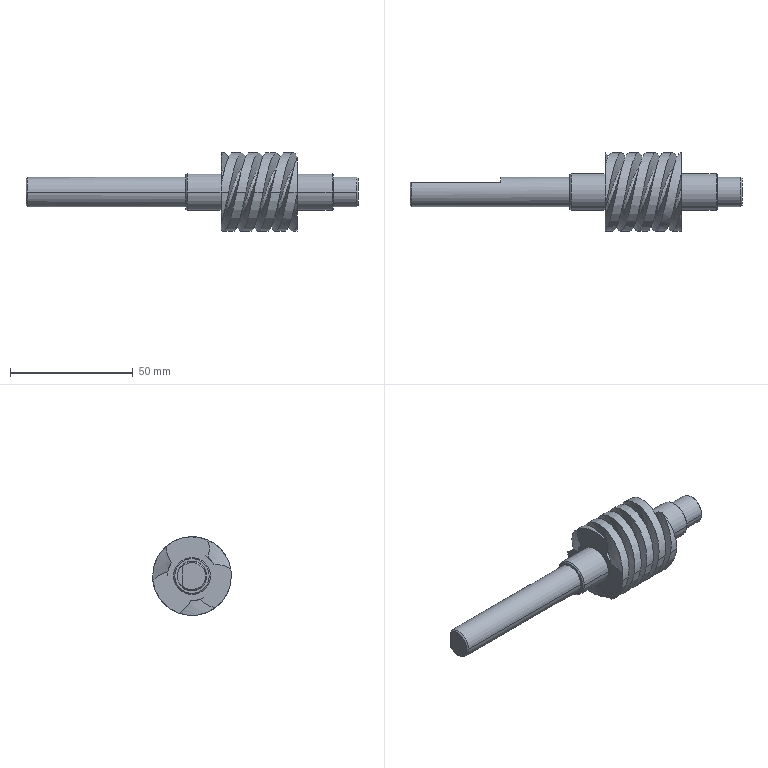Part | SolidWorks | features ICE 3, Chamfer 1, CirPattern 1, Helix 1, Revolution 1, SweepCut 1 | 1 solid | 45 faces | box 135 x 31.98 x 31.98 mm | volume 33052 mm3 | cylinder 21 | spline 9 | plane 8 | cone 7 | commonest cylinder face diameters 31.98 x13 12 x4 15 x4